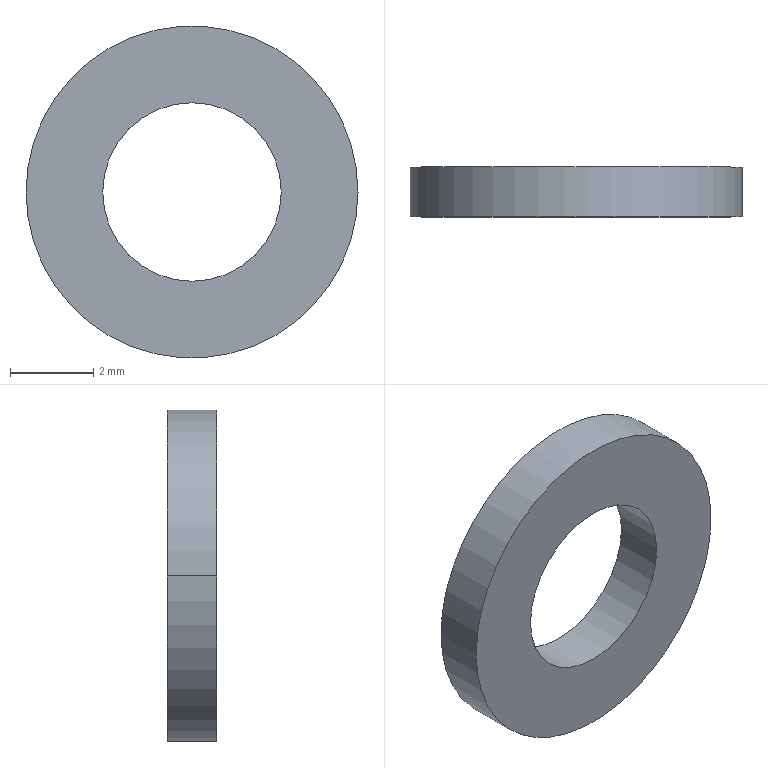Part | STEP file | WSX-SUS-M4X8-1.2-12 | 1 solid | 6 faces | box 8 x 1.2 x 8 mm | volume 42.892 mm3 | cylinder 4 | plane 2 | commonest cylinder face diameters 4.3 x2 8 x2
STEP:
#1=CARTESIAN_POINT('',(2.15,0.,0.));
#2=VERTEX_POINT('',#1);
#3=CARTESIAN_POINT('',(-2.15,0.,0.));
#4=VERTEX_POINT('',#3);
#5=CARTESIAN_POINT('',(0.,0.,0.));
#6=DIRECTION('',(0.,1.,0.));
#7=DIRECTION('',(-1.,0.,0.));
#8=AXIS2_PLACEMENT_3D('',#5,#6,#7);
#9=CIRCLE('',#8,2.15);
#10=EDGE_CURVE('',#2,#4,#9,.T.);
#11=ORIENTED_EDGE('',*,*,#10,.F.);
#12=CARTESIAN_POINT('',(2.15,1.2,0.));
#13=VERTEX_POINT('',#12);
#14=CARTESIAN_POINT('',(2.15,0.,0.));
#15=DIRECTION('',(0.,1.,0.));
#16=VECTOR('',#15,1000.);
#17=LINE('',#14,#16);
#18=EDGE_CURVE('',#2,#13,#17,.T.);
#19=ORIENTED_EDGE('',*,*,#18,.T.);
#20=CARTESIAN_POINT('',(-2.15,1.2,0.));
#21=VERTEX_POINT('',#20);
#22=CARTESIAN_POINT('',(0.,1.2,0.));
#23=DIRECTION('',(0.,-1.,0.));
#24=DIRECTION('',(1.,0.,0.));
#25=AXIS2_PLACEMENT_3D('',#22,#23,#24);
#26=CIRCLE('',#25,2.15);
#27=EDGE_CURVE('',#21,#13,#26,.T.);
#28=ORIENTED_EDGE('',*,*,#27,.F.);
#29=CARTESIAN_POINT('',(-2.15,0.,0.));
#30=DIRECTION('',(0.,1.,0.));
#31=VECTOR('',#30,1000.);
#32=LINE('',#29,#31);
#33=EDGE_CURVE('',#4,#21,#32,.T.);
#34=ORIENTED_EDGE('',*,*,#33,.F.);
#35=EDGE_LOOP('',(#11,#19,#28,#34));
#36=FACE_OUTER_BOUND('',#35,.T.);
#37=CARTESIAN_POINT('',(0.,0.,0.));
#38=DIRECTION('',(0.,1.,0.));
#39=DIRECTION('',(-1.,0.,0.));
#40=AXIS2_PLACEMENT_3D('',#37,#38,#39);
#41=CYLINDRICAL_SURFACE('',#40,2.15);
#42=ADVANCED_FACE('',(#36),#41,.F.);
#43=CARTESIAN_POINT('',(-4.,0.,0.));
#44=VERTEX_POINT('',#43);
#45=CARTESIAN_POINT('',(4.,0.,0.));
#46=VERTEX_POINT('',#45);
#47=CARTESIAN_POINT('',(0.,0.,0.));
#48=DIRECTION('',(0.,1.,0.));
#49=DIRECTION('',(-1.,0.,0.));
#50=AXIS2_PLACEMENT_3D('',#47,#48,#49);
#51=CIRCLE('',#50,4.);
#52=EDGE_CURVE('',#44,#46,#51,.T.);
#53=ORIENTED_EDGE('',*,*,#52,.T.);
#54=CARTESIAN_POINT('',(4.,1.2,0.));
#55=VERTEX_POINT('',#54);
#56=CARTESIAN_POINT('',(4.,0.,0.));
#57=DIRECTION('',(0.,1.,0.));
#58=VECTOR('',#57,1000.);
#59=LINE('',#56,#58);
#60=EDGE_CURVE('',#46,#55,#59,.T.);
#61=ORIENTED_EDGE('',*,*,#60,.T.);
#62=CARTESIAN_POINT('',(-4.,1.2,0.));
#63=VERTEX_POINT('',#62);
#64=CARTESIAN_POINT('',(0.,1.2,0.));
#65=DIRECTION('',(0.,-1.,0.));
#66=DIRECTION('',(1.,0.,0.));
#67=AXIS2_PLACEMENT_3D('',#64,#65,#66);
#68=CIRCLE('',#67,4.);
#69=EDGE_CURVE('',#55,#63,#68,.T.);
#70=ORIENTED_EDGE('',*,*,#69,.T.);
#71=CARTESIAN_POINT('',(-4.,0.,0.));
#72=DIRECTION('',(0.,1.,0.));
#73=VECTOR('',#72,1000.);
#74=LINE('',#71,#73);
#75=EDGE_CURVE('',#44,#63,#74,.T.);
#76=ORIENTED_EDGE('',*,*,#75,.F.);
#77=EDGE_LOOP('',(#53,#61,#70,#76));
#78=FACE_OUTER_BOUND('',#77,.T.);
#79=CARTESIAN_POINT('',(0.,0.,0.));
#80=DIRECTION('',(0.,1.,0.));
#81=DIRECTION('',(-1.,0.,0.));
#82=AXIS2_PLACEMENT_3D('',#79,#80,#81);
#83=CYLINDRICAL_SURFACE('',#82,4.);
#84=ADVANCED_FACE('',(#78),#83,.T.);
#85=ORIENTED_EDGE('',*,*,#27,.T.);
#86=CARTESIAN_POINT('',(0.,1.2,0.));
#87=DIRECTION('',(0.,-1.,0.));
#88=DIRECTION('',(1.,0.,0.));
#89=AXIS2_PLACEMENT_3D('',#86,#87,#88);
#90=CIRCLE('',#89,2.15);
#91=EDGE_CURVE('',#13,#21,#90,.T.);
#92=ORIENTED_EDGE('',*,*,#91,.T.);
#93=EDGE_LOOP('',(#85,#92));
#94=FACE_BOUND('',#93,.T.);
#95=CARTESIAN_POINT('',(0.,1.2,0.));
#96=DIRECTION('',(0.,-1.,0.));
#97=DIRECTION('',(1.,0.,0.));
#98=AXIS2_PLACEMENT_3D('',#95,#96,#97);
#99=CIRCLE('',#98,4.);
#100=EDGE_CURVE('',#63,#55,#99,.T.);
#101=ORIENTED_EDGE('',*,*,#100,.F.);
#102=ORIENTED_EDGE('',*,*,#69,.F.);
#103=EDGE_LOOP('',(#101,#102));
#104=FACE_OUTER_BOUND('',#103,.T.);
#105=CARTESIAN_POINT('',(0.,1.2,0.));
#106=DIRECTION('',(0.,1.,0.));
#107=DIRECTION('',(-1.,0.,0.));
#108=AXIS2_PLACEMENT_3D('',#105,#106,#107);
#109=PLANE('',#108);
#110=ADVANCED_FACE('',(#94,#104),#109,.T.);
#111=CARTESIAN_POINT('',(0.,0.,0.));
#112=DIRECTION('',(0.,1.,0.));
#113=DIRECTION('',(-1.,0.,0.));
#114=AXIS2_PLACEMENT_3D('',#111,#112,#113);
#115=CIRCLE('',#114,2.15);
#116=EDGE_CURVE('',#4,#2,#115,.T.);
#117=ORIENTED_EDGE('',*,*,#116,.T.);
#118=ORIENTED_EDGE('',*,*,#10,.T.);
#119=EDGE_LOOP('',(#117,#118));
#120=FACE_BOUND('',#119,.T.);
#121=ORIENTED_EDGE('',*,*,#52,.F.);
#122=CARTESIAN_POINT('',(0.,0.,0.));
#123=DIRECTION('',(0.,1.,0.));
#124=DIRECTION('',(-1.,0.,0.));
#125=AXIS2_PLACEMENT_3D('',#122,#123,#124);
#126=CIRCLE('',#125,4.);
#127=EDGE_CURVE('',#46,#44,#126,.T.);
#128=ORIENTED_EDGE('',*,*,#127,.F.);
#129=EDGE_LOOP('',(#121,#128));
#130=FACE_OUTER_BOUND('',#129,.T.);
#131=CARTESIAN_POINT('',(0.,0.,0.));
#132=DIRECTION('',(0.,-1.,0.));
#133=DIRECTION('',(1.,0.,0.));
#134=AXIS2_PLACEMENT_3D('',#131,#132,#133);
#135=PLANE('',#134);
#136=ADVANCED_FACE('',(#120,#130),#135,.T.);
#137=ORIENTED_EDGE('',*,*,#60,.F.);
#138=ORIENTED_EDGE('',*,*,#127,.T.);
#139=ORIENTED_EDGE('',*,*,#75,.T.);
#140=ORIENTED_EDGE('',*,*,#100,.T.);
#141=EDGE_LOOP('',(#137,#138,#139,#140));
#142=FACE_OUTER_BOUND('',#141,.T.);
#143=CARTESIAN_POINT('',(0.,0.,0.));
#144=DIRECTION('',(0.,1.,0.));
#145=DIRECTION('',(-1.,0.,0.));
#146=AXIS2_PLACEMENT_3D('',#143,#144,#145);
#147=CYLINDRICAL_SURFACE('',#146,4.);
#148=ADVANCED_FACE('',(#142),#147,.T.);
#149=ORIENTED_EDGE('',*,*,#18,.F.);
#150=ORIENTED_EDGE('',*,*,#116,.F.);
#151=ORIENTED_EDGE('',*,*,#33,.T.);
#152=ORIENTED_EDGE('',*,*,#91,.F.);
#153=EDGE_LOOP('',(#149,#150,#151,#152));
#154=FACE_OUTER_BOUND('',#153,.T.);
#155=CARTESIAN_POINT('',(0.,0.,0.));
#156=DIRECTION('',(0.,1.,0.));
#157=DIRECTION('',(-1.,0.,0.));
#158=AXIS2_PLACEMENT_3D('',#155,#156,#157);
#159=CYLINDRICAL_SURFACE('',#158,2.15);
#160=ADVANCED_FACE('',(#154),#159,.F.);
#161=CLOSED_SHELL('',(#42,#84,#110,#136,#148,#160));
#162=MANIFOLD_SOLID_BREP('',#161);
#163=CARTESIAN_POINT('',(0.,0.,0.));
#164=DIRECTION('',(0.,0.,1.));
#165=DIRECTION('',(1.,0.,0.));
#166=AXIS2_PLACEMENT_3D('',#163,#164,#165);
#167=(LENGTH_UNIT()NAMED_UNIT(*)SI_UNIT(.MILLI.,.METRE.));
#168=UNCERTAINTY_MEASURE_WITH_UNIT(LENGTH_MEASURE(0.00001),#167,'','');
#169=(NAMED_UNIT(*)PLANE_ANGLE_UNIT()SI_UNIT($,.RADIAN.));
#170=(NAMED_UNIT(*)SI_UNIT($,.STERADIAN.)SOLID_ANGLE_UNIT());
#171=(GEOMETRIC_REPRESENTATION_CONTEXT(3)GLOBAL_UNCERTAINTY_ASSIGNED_CONTEXT((#168))GLOBAL_UNIT_ASSIGNED_CONTEXT((#167,#169,#170))REPRESENTATION_CONTEXT('',''));
#172=ADVANCED_BREP_SHAPE_REPRESENTATION('',(#162,#166),#171);